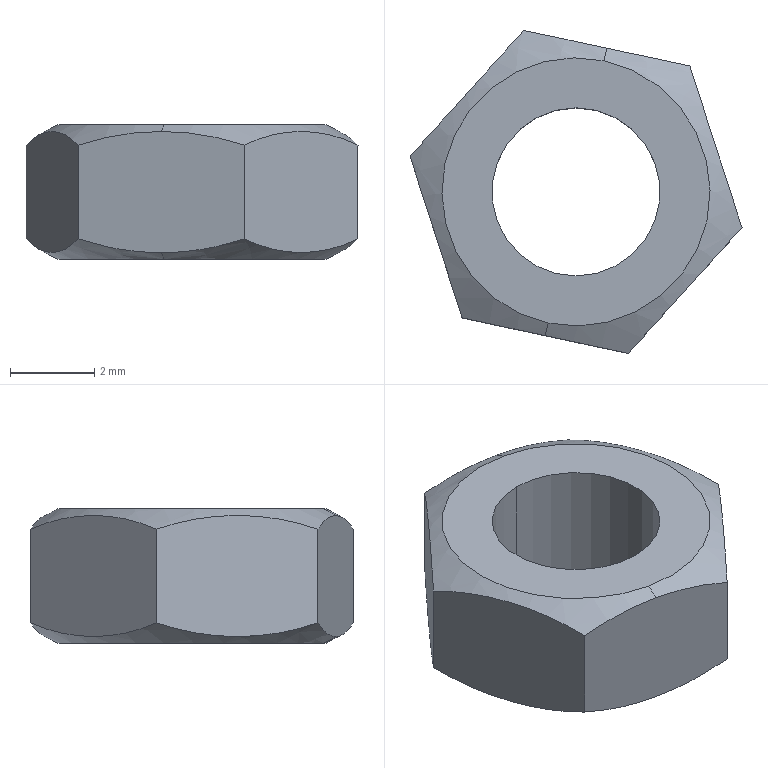Part | STEP file | MSBR-12_1_1_1_1 | 1 solid | 14 faces | box 7.904 x 7.691 x 3.2 mm | volume 92.564 mm3 | plane 8 | sphere 4 | cylinder 2 | commonest cylinder face diameters 4 x2
STEP:
#1=CARTESIAN_POINT('',(0.,0.,0.));
#2=DIRECTION('',(0.,0.,1.));
#3=DIRECTION('',(1.,0.,0.));
#4=AXIS2_PLACEMENT_3D('',#1,#2,#3);
#5=CARTESIAN_POINT('',(-32.173,30.173,38.8));
#6=VERTEX_POINT('',#5);
#7=CARTESIAN_POINT('',(-32.173,30.173,35.6));
#8=VERTEX_POINT('',#7);
#9=CARTESIAN_POINT('',(-32.173,30.173,38.8));
#10=DIRECTION('',(0.,0.,-1.));
#11=VECTOR('',#10,3.2);
#12=LINE('',#9,#11);
#13=EDGE_CURVE('',#6,#8,#12,.T.);
#14=ORIENTED_EDGE('',*,*,#13,.F.);
#15=CARTESIAN_POINT('',(-32.173,34.173,38.8));
#16=VERTEX_POINT('',#15);
#17=CARTESIAN_POINT('',(-32.173,32.173,38.8));
#18=DIRECTION('',(0.,0.,1.));
#19=DIRECTION('',(0.,1.,0.));
#20=AXIS2_PLACEMENT_3D('',#17,#18,#19);
#21=CIRCLE('',#20,2.);
#22=EDGE_CURVE('',#16,#6,#21,.T.);
#23=ORIENTED_EDGE('',*,*,#22,.F.);
#24=CARTESIAN_POINT('',(-32.173,34.173,35.6));
#25=VERTEX_POINT('',#24);
#26=CARTESIAN_POINT('',(-32.173,34.173,35.6));
#27=DIRECTION('',(0.,0.,1.));
#28=VECTOR('',#27,3.2);
#29=LINE('',#26,#28);
#30=EDGE_CURVE('',#25,#16,#29,.T.);
#31=ORIENTED_EDGE('',*,*,#30,.F.);
#32=CARTESIAN_POINT('',(-32.173,32.173,35.6));
#33=DIRECTION('',(0.,0.,-1.));
#34=DIRECTION('',(0.,-1.,0.));
#35=AXIS2_PLACEMENT_3D('',#32,#33,#34);
#36=CIRCLE('',#35,2.);
#37=EDGE_CURVE('',#8,#25,#36,.T.);
#38=ORIENTED_EDGE('',*,*,#37,.F.);
#39=EDGE_LOOP('',(#14,#23,#31,#38));
#40=FACE_OUTER_BOUND('',#39,.F.);
#41=CARTESIAN_POINT('',(-32.173,32.173,35.536));
#42=DIRECTION('',(0.,0.,1.));
#43=DIRECTION('',(0.,1.,0.));
#44=AXIS2_PLACEMENT_3D('',#41,#42,#43);
#45=CYLINDRICAL_SURFACE('',#44,2.);
#46=ADVANCED_FACE('',(#40),#45,.F.);
#47=CARTESIAN_POINT('',(-32.173,32.173,38.8));
#48=DIRECTION('',(0.,0.,1.));
#49=DIRECTION('',(0.,-1.,0.));
#50=AXIS2_PLACEMENT_3D('',#47,#48,#49);
#51=CIRCLE('',#50,2.);
#52=EDGE_CURVE('',#6,#16,#51,.T.);
#53=ORIENTED_EDGE('',*,*,#52,.F.);
#54=ORIENTED_EDGE('',*,*,#13,.T.);
#55=CARTESIAN_POINT('',(-32.173,32.173,35.6));
#56=DIRECTION('',(0.,0.,-1.));
#57=DIRECTION('',(0.,1.,0.));
#58=AXIS2_PLACEMENT_3D('',#55,#56,#57);
#59=CIRCLE('',#58,2.);
#60=EDGE_CURVE('',#25,#8,#59,.T.);
#61=ORIENTED_EDGE('',*,*,#60,.F.);
#62=ORIENTED_EDGE('',*,*,#30,.T.);
#63=EDGE_LOOP('',(#53,#54,#61,#62));
#64=FACE_OUTER_BOUND('',#63,.F.);
#65=CARTESIAN_POINT('',(-32.173,32.173,35.536));
#66=DIRECTION('',(0.,0.,1.));
#67=DIRECTION('',(0.,-1.,0.));
#68=AXIS2_PLACEMENT_3D('',#65,#66,#67);
#69=CYLINDRICAL_SURFACE('',#68,2.);
#70=ADVANCED_FACE('',(#64),#69,.F.);
#71=CARTESIAN_POINT('',(-32.842,29.052,38.8));
#72=VERTEX_POINT('',#71);
#73=CARTESIAN_POINT('',(-31.505,35.295,38.8));
#74=VERTEX_POINT('',#73);
#75=CARTESIAN_POINT('',(-32.173,32.173,38.8));
#76=DIRECTION('',(0.,0.,1.));
#77=DIRECTION('',(-0.2094,-0.9778,0.));
#78=AXIS2_PLACEMENT_3D('',#75,#76,#77);
#79=CIRCLE('',#78,3.192);
#80=EDGE_CURVE('',#72,#74,#79,.T.);
#81=ORIENTED_EDGE('',*,*,#80,.F.);
#82=CARTESIAN_POINT('',(-32.173,32.173,38.8));
#83=DIRECTION('',(0.,0.,-1.));
#84=DIRECTION('',(-0.2094,-0.9778,0.));
#85=AXIS2_PLACEMENT_3D('',#82,#83,#84);
#86=CIRCLE('',#85,3.192);
#87=EDGE_CURVE('',#72,#74,#86,.T.);
#88=ORIENTED_EDGE('',*,*,#87,.T.);
#89=EDGE_LOOP('',(#81,#88));
#90=FACE_OUTER_BOUND('',#89,.F.);
#91=ORIENTED_EDGE('',*,*,#22,.T.);
#92=ORIENTED_EDGE('',*,*,#52,.T.);
#93=EDGE_LOOP('',(#91,#92));
#94=FACE_BOUND('',#93,.F.);
#95=CARTESIAN_POINT('',(-32.173,32.173,38.8));
#96=DIRECTION('',(0.,0.,1.));
#97=DIRECTION('',(0.9778,-0.2094,0.));
#98=AXIS2_PLACEMENT_3D('',#95,#96,#97);
#99=PLANE('',#98);
#100=ADVANCED_FACE('',(#90,#94),#99,.T.);
#101=CARTESIAN_POINT('',(-32.906,28.751,38.641));
#102=VERTEX_POINT('',#101);
#103=CARTESIAN_POINT('',(-32.173,32.173,32.235));
#104=DIRECTION('',(0.9778,-0.2094,-0.000000001));
#105=DIRECTION('',(-0.09156,-0.4276,0.8993));
#106=AXIS2_PLACEMENT_3D('',#103,#104,#105);
#107=CIRCLE('',#106,7.3);
#108=EDGE_CURVE('',#72,#102,#107,.T.);
#109=ORIENTED_EDGE('',*,*,#108,.F.);
#110=ORIENTED_EDGE('',*,*,#80,.T.);
#111=CARTESIAN_POINT('',(-31.44,35.596,38.641));
#112=VERTEX_POINT('',#111);
#113=CARTESIAN_POINT('',(-32.173,32.173,32.235));
#114=DIRECTION('',(0.9778,-0.2094,-0.000000001));
#115=DIRECTION('',(0.1004,0.4688,0.8776));
#116=AXIS2_PLACEMENT_3D('',#113,#114,#115);
#117=CIRCLE('',#116,7.3);
#118=EDGE_CURVE('',#112,#74,#117,.T.);
#119=ORIENTED_EDGE('',*,*,#118,.F.);
#120=CARTESIAN_POINT('',(-29.465,35.173,38.314));
#121=VERTEX_POINT('',#120);
#122=CARTESIAN_POINT('',(-31.44,35.596,32.235));
#123=DIRECTION('',(0.2094,0.9778,0.));
#124=DIRECTION('',(-0.000000002,0.,1.));
#125=AXIS2_PLACEMENT_3D('',#122,#123,#124);
#126=CIRCLE('',#125,6.406);
#127=EDGE_CURVE('',#112,#121,#126,.T.);
#128=ORIENTED_EDGE('',*,*,#127,.T.);
#129=CARTESIAN_POINT('',(-28.222,31.327,38.314));
#130=VERTEX_POINT('',#129);
#131=CARTESIAN_POINT('',(-28.843,33.25,32.235));
#132=DIRECTION('',(0.9515,0.3076,0.));
#133=DIRECTION('',(-0.09701,0.3001,0.9489));
#134=AXIS2_PLACEMENT_3D('',#131,#132,#133);
#135=CIRCLE('',#134,6.406);
#136=EDGE_CURVE('',#121,#130,#135,.T.);
#137=ORIENTED_EDGE('',*,*,#136,.T.);
#138=CARTESIAN_POINT('',(-30.93,28.328,38.314));
#139=VERTEX_POINT('',#138);
#140=CARTESIAN_POINT('',(-29.576,29.827,32.235));
#141=DIRECTION('',(0.7421,-0.6703,0.));
#142=DIRECTION('',(0.2114,0.2341,0.9489));
#143=AXIS2_PLACEMENT_3D('',#140,#141,#142);
#144=CIRCLE('',#143,6.406);
#145=EDGE_CURVE('',#130,#139,#144,.T.);
#146=ORIENTED_EDGE('',*,*,#145,.T.);
#147=CARTESIAN_POINT('',(-32.906,28.751,32.235));
#148=DIRECTION('',(0.2094,0.9778,0.));
#149=DIRECTION('',(-0.000000001,0.,1.));
#150=AXIS2_PLACEMENT_3D('',#147,#148,#149);
#151=CIRCLE('',#150,6.406);
#152=EDGE_CURVE('',#102,#139,#151,.T.);
#153=ORIENTED_EDGE('',*,*,#152,.F.);
#154=EDGE_LOOP('',(#109,#110,#119,#128,#137,#146,#153));
#155=FACE_OUTER_BOUND('',#154,.F.);
#156=CARTESIAN_POINT('',(-32.173,32.173,32.235));
#157=DIRECTION('',(0.09156,0.4276,0.8993));
#158=DIRECTION('',(-0.1883,-0.8794,0.4373));
#159=AXIS2_PLACEMENT_3D('',#156,#157,#158);
#160=SPHERICAL_SURFACE('',#159,7.3);
#161=ADVANCED_FACE('',(#155),#160,.T.);
#162=CARTESIAN_POINT('',(-34.882,29.174,38.314));
#163=VERTEX_POINT('',#162);
#164=CARTESIAN_POINT('',(-32.906,28.751,32.235));
#165=DIRECTION('',(0.2094,0.9778,0.));
#166=DIRECTION('',(-0.3084,0.06605,0.9489));
#167=AXIS2_PLACEMENT_3D('',#164,#165,#166);
#168=CIRCLE('',#167,6.406);
#169=EDGE_CURVE('',#163,#102,#168,.T.);
#170=ORIENTED_EDGE('',*,*,#169,.F.);
#171=CARTESIAN_POINT('',(-36.125,33.02,38.314));
#172=VERTEX_POINT('',#171);
#173=CARTESIAN_POINT('',(-35.504,31.097,32.235));
#174=DIRECTION('',(-0.9515,-0.3076,0.));
#175=DIRECTION('',(0.09701,-0.3001,0.9489));
#176=AXIS2_PLACEMENT_3D('',#173,#174,#175);
#177=CIRCLE('',#176,6.406);
#178=EDGE_CURVE('',#163,#172,#177,.T.);
#179=ORIENTED_EDGE('',*,*,#178,.T.);
#180=CARTESIAN_POINT('',(-33.416,36.019,38.314));
#181=VERTEX_POINT('',#180);
#182=CARTESIAN_POINT('',(-34.771,34.519,32.235));
#183=DIRECTION('',(-0.7421,0.6703,0.));
#184=DIRECTION('',(-0.2114,-0.2341,0.9489));
#185=AXIS2_PLACEMENT_3D('',#182,#183,#184);
#186=CIRCLE('',#185,6.406);
#187=EDGE_CURVE('',#172,#181,#186,.T.);
#188=ORIENTED_EDGE('',*,*,#187,.T.);
#189=CARTESIAN_POINT('',(-31.44,35.596,32.235));
#190=DIRECTION('',(0.2094,0.9778,0.));
#191=DIRECTION('',(-0.3084,0.06605,0.9489));
#192=AXIS2_PLACEMENT_3D('',#189,#190,#191);
#193=CIRCLE('',#192,6.406);
#194=EDGE_CURVE('',#181,#112,#193,.T.);
#195=ORIENTED_EDGE('',*,*,#194,.T.);
#196=ORIENTED_EDGE('',*,*,#118,.T.);
#197=ORIENTED_EDGE('',*,*,#87,.F.);
#198=ORIENTED_EDGE('',*,*,#108,.T.);
#199=EDGE_LOOP('',(#170,#179,#188,#195,#196,#197,#198));
#200=FACE_OUTER_BOUND('',#199,.F.);
#201=CARTESIAN_POINT('',(-32.173,32.173,32.235));
#202=DIRECTION('',(0.09156,0.4276,0.8993));
#203=DIRECTION('',(0.1883,0.8794,-0.4373));
#204=AXIS2_PLACEMENT_3D('',#201,#202,#203);
#205=SPHERICAL_SURFACE('',#204,7.3);
#206=ADVANCED_FACE('',(#200),#205,.T.);
#207=ORIENTED_EDGE('',*,*,#152,.T.);
#208=CARTESIAN_POINT('',(-30.93,28.328,36.086));
#209=VERTEX_POINT('',#208);
#210=CARTESIAN_POINT('',(-30.93,28.328,36.086));
#211=DIRECTION('',(0.,0.,1.));
#212=VECTOR('',#211,2.228);
#213=LINE('',#210,#212);
#214=EDGE_CURVE('',#209,#139,#213,.T.);
#215=ORIENTED_EDGE('',*,*,#214,.F.);
#216=CARTESIAN_POINT('',(-32.906,28.751,35.759));
#217=VERTEX_POINT('',#216);
#218=CARTESIAN_POINT('',(-32.906,28.751,42.165));
#219=DIRECTION('',(-0.2094,-0.9778,0.));
#220=DIRECTION('',(-0.000000001,0.,-1.));
#221=AXIS2_PLACEMENT_3D('',#218,#219,#220);
#222=CIRCLE('',#221,6.406);
#223=EDGE_CURVE('',#217,#209,#222,.T.);
#224=ORIENTED_EDGE('',*,*,#223,.F.);
#225=CARTESIAN_POINT('',(-34.882,29.174,36.086));
#226=VERTEX_POINT('',#225);
#227=CARTESIAN_POINT('',(-32.906,28.751,42.165));
#228=DIRECTION('',(-0.2094,-0.9778,0.));
#229=DIRECTION('',(-0.3084,0.06605,-0.9489));
#230=AXIS2_PLACEMENT_3D('',#227,#228,#229);
#231=CIRCLE('',#230,6.406);
#232=EDGE_CURVE('',#226,#217,#231,.T.);
#233=ORIENTED_EDGE('',*,*,#232,.F.);
#234=CARTESIAN_POINT('',(-34.882,29.174,38.314));
#235=DIRECTION('',(0.,0.,-1.));
#236=VECTOR('',#235,2.228);
#237=LINE('',#234,#236);
#238=EDGE_CURVE('',#163,#226,#237,.T.);
#239=ORIENTED_EDGE('',*,*,#238,.F.);
#240=ORIENTED_EDGE('',*,*,#169,.T.);
#241=EDGE_LOOP('',(#207,#215,#224,#233,#239,#240));
#242=FACE_OUTER_BOUND('',#241,.F.);
#243=CARTESIAN_POINT('',(-32.906,28.751,37.2));
#244=DIRECTION('',(0.2094,0.9778,0.));
#245=DIRECTION('',(0.9778,-0.2094,0.));
#246=AXIS2_PLACEMENT_3D('',#243,#244,#245);
#247=PLANE('',#246);
#248=ADVANCED_FACE('',(#242),#247,.F.);
#249=ORIENTED_EDGE('',*,*,#145,.F.);
#250=CARTESIAN_POINT('',(-28.222,31.327,36.086));
#251=VERTEX_POINT('',#250);
#252=CARTESIAN_POINT('',(-28.222,31.327,36.086));
#253=DIRECTION('',(0.,0.,1.));
#254=VECTOR('',#253,2.228);
#255=LINE('',#252,#254);
#256=EDGE_CURVE('',#251,#130,#255,.T.);
#257=ORIENTED_EDGE('',*,*,#256,.F.);
#258=CARTESIAN_POINT('',(-29.576,29.827,42.165));
#259=DIRECTION('',(0.7421,-0.6703,0.));
#260=DIRECTION('',(-0.2114,-0.2341,-0.9489));
#261=AXIS2_PLACEMENT_3D('',#258,#259,#260);
#262=CIRCLE('',#261,6.406);
#263=EDGE_CURVE('',#209,#251,#262,.T.);
#264=ORIENTED_EDGE('',*,*,#263,.F.);
#265=ORIENTED_EDGE('',*,*,#214,.T.);
#266=EDGE_LOOP('',(#249,#257,#264,#265));
#267=FACE_OUTER_BOUND('',#266,.F.);
#268=CARTESIAN_POINT('',(-29.576,29.827,37.2));
#269=DIRECTION('',(0.7421,-0.6703,0.));
#270=DIRECTION('',(0.6703,0.7421,0.));
#271=AXIS2_PLACEMENT_3D('',#268,#269,#270);
#272=PLANE('',#271);
#273=ADVANCED_FACE('',(#267),#272,.T.);
#274=ORIENTED_EDGE('',*,*,#136,.F.);
#275=CARTESIAN_POINT('',(-29.465,35.173,36.086));
#276=VERTEX_POINT('',#275);
#277=CARTESIAN_POINT('',(-29.465,35.173,36.086));
#278=DIRECTION('',(0.,0.,1.));
#279=VECTOR('',#278,2.228);
#280=LINE('',#277,#279);
#281=EDGE_CURVE('',#276,#121,#280,.T.);
#282=ORIENTED_EDGE('',*,*,#281,.F.);
#283=CARTESIAN_POINT('',(-28.843,33.25,42.165));
#284=DIRECTION('',(0.9515,0.3076,0.));
#285=DIRECTION('',(0.09701,-0.3001,-0.9489));
#286=AXIS2_PLACEMENT_3D('',#283,#284,#285);
#287=CIRCLE('',#286,6.406);
#288=EDGE_CURVE('',#251,#276,#287,.T.);
#289=ORIENTED_EDGE('',*,*,#288,.F.);
#290=ORIENTED_EDGE('',*,*,#256,.T.);
#291=EDGE_LOOP('',(#274,#282,#289,#290));
#292=FACE_OUTER_BOUND('',#291,.F.);
#293=CARTESIAN_POINT('',(-28.843,33.25,37.2));
#294=DIRECTION('',(0.9515,0.3076,0.));
#295=DIRECTION('',(-0.3076,0.9515,0.));
#296=AXIS2_PLACEMENT_3D('',#293,#294,#295);
#297=PLANE('',#296);
#298=ADVANCED_FACE('',(#292),#297,.T.);
#299=ORIENTED_EDGE('',*,*,#281,.T.);
#300=ORIENTED_EDGE('',*,*,#127,.F.);
#301=ORIENTED_EDGE('',*,*,#194,.F.);
#302=CARTESIAN_POINT('',(-33.416,36.019,36.086));
#303=VERTEX_POINT('',#302);
#304=CARTESIAN_POINT('',(-33.416,36.019,36.086));
#305=DIRECTION('',(0.,0.,1.));
#306=VECTOR('',#305,2.228);
#307=LINE('',#304,#306);
#308=EDGE_CURVE('',#303,#181,#307,.T.);
#309=ORIENTED_EDGE('',*,*,#308,.F.);
#310=CARTESIAN_POINT('',(-31.44,35.596,35.759));
#311=VERTEX_POINT('',#310);
#312=CARTESIAN_POINT('',(-31.44,35.596,42.165));
#313=DIRECTION('',(-0.2094,-0.9778,0.));
#314=DIRECTION('',(-0.3084,0.06605,-0.9489));
#315=AXIS2_PLACEMENT_3D('',#312,#313,#314);
#316=CIRCLE('',#315,6.406);
#317=EDGE_CURVE('',#303,#311,#316,.T.);
#318=ORIENTED_EDGE('',*,*,#317,.T.);
#319=CARTESIAN_POINT('',(-31.44,35.596,42.165));
#320=DIRECTION('',(-0.2094,-0.9778,0.));
#321=DIRECTION('',(-0.000000001,0.,-1.));
#322=AXIS2_PLACEMENT_3D('',#319,#320,#321);
#323=CIRCLE('',#322,6.406);
#324=EDGE_CURVE('',#311,#276,#323,.T.);
#325=ORIENTED_EDGE('',*,*,#324,.T.);
#326=EDGE_LOOP('',(#299,#300,#301,#309,#318,#325));
#327=FACE_OUTER_BOUND('',#326,.F.);
#328=CARTESIAN_POINT('',(-31.44,35.596,37.2));
#329=DIRECTION('',(0.2094,0.9778,0.));
#330=DIRECTION('',(-0.9778,0.2094,0.));
#331=AXIS2_PLACEMENT_3D('',#328,#329,#330);
#332=PLANE('',#331);
#333=ADVANCED_FACE('',(#327),#332,.T.);
#334=CARTESIAN_POINT('',(-36.125,33.02,36.086));
#335=VERTEX_POINT('',#334);
#336=CARTESIAN_POINT('',(-34.771,34.519,42.165));
#337=DIRECTION('',(-0.7421,0.6703,0.));
#338=DIRECTION('',(0.2114,0.2341,-0.9489));
#339=AXIS2_PLACEMENT_3D('',#336,#337,#338);
#340=CIRCLE('',#339,6.406);
#341=EDGE_CURVE('',#303,#335,#340,.T.);
#342=ORIENTED_EDGE('',*,*,#341,.F.);
#343=ORIENTED_EDGE('',*,*,#308,.T.);
#344=ORIENTED_EDGE('',*,*,#187,.F.);
#345=CARTESIAN_POINT('',(-36.125,33.02,36.086));
#346=DIRECTION('',(0.,0.,1.));
#347=VECTOR('',#346,2.228);
#348=LINE('',#345,#347);
#349=EDGE_CURVE('',#335,#172,#348,.T.);
#350=ORIENTED_EDGE('',*,*,#349,.F.);
#351=EDGE_LOOP('',(#342,#343,#344,#350));
#352=FACE_OUTER_BOUND('',#351,.F.);
#353=CARTESIAN_POINT('',(-34.771,34.519,37.2));
#354=DIRECTION('',(0.7421,-0.6703,0.));
#355=DIRECTION('',(-0.6703,-0.7421,0.));
#356=AXIS2_PLACEMENT_3D('',#353,#354,#355);
#357=PLANE('',#356);
#358=ADVANCED_FACE('',(#352),#357,.F.);
#359=CARTESIAN_POINT('',(-32.842,29.052,35.6));
#360=VERTEX_POINT('',#359);
#361=CARTESIAN_POINT('',(-31.505,35.295,35.6));
#362=VERTEX_POINT('',#361);
#363=CARTESIAN_POINT('',(-32.173,32.173,35.6));
#364=DIRECTION('',(0.,0.,-1.));
#365=DIRECTION('',(-0.2094,-0.9778,0.));
#366=AXIS2_PLACEMENT_3D('',#363,#364,#365);
#367=CIRCLE('',#366,3.192);
#368=EDGE_CURVE('',#360,#362,#367,.T.);
#369=ORIENTED_EDGE('',*,*,#368,.T.);
#370=CARTESIAN_POINT('',(-32.173,32.173,42.165));
#371=DIRECTION('',(-0.9778,0.2094,0.000000001));
#372=DIRECTION('',(0.1004,0.4688,-0.8776));
#373=AXIS2_PLACEMENT_3D('',#370,#371,#372);
#374=CIRCLE('',#373,7.3);
#375=EDGE_CURVE('',#311,#362,#374,.T.);
#376=ORIENTED_EDGE('',*,*,#375,.F.);
#377=ORIENTED_EDGE('',*,*,#317,.F.);
#378=ORIENTED_EDGE('',*,*,#341,.T.);
#379=CARTESIAN_POINT('',(-35.504,31.097,42.165));
#380=DIRECTION('',(-0.9515,-0.3076,0.));
#381=DIRECTION('',(-0.09701,0.3001,-0.9489));
#382=AXIS2_PLACEMENT_3D('',#379,#380,#381);
#383=CIRCLE('',#382,6.406);
#384=EDGE_CURVE('',#335,#226,#383,.T.);
#385=ORIENTED_EDGE('',*,*,#384,.T.);
#386=ORIENTED_EDGE('',*,*,#232,.T.);
#387=CARTESIAN_POINT('',(-32.173,32.173,42.165));
#388=DIRECTION('',(-0.9778,0.2094,0.000000005));
#389=DIRECTION('',(-0.09156,-0.4276,-0.8993));
#390=AXIS2_PLACEMENT_3D('',#387,#388,#389);
#391=CIRCLE('',#390,7.3);
#392=EDGE_CURVE('',#360,#217,#391,.T.);
#393=ORIENTED_EDGE('',*,*,#392,.F.);
#394=EDGE_LOOP('',(#369,#376,#377,#378,#385,#386,#393));
#395=FACE_OUTER_BOUND('',#394,.F.);
#396=CARTESIAN_POINT('',(-32.173,32.173,42.165));
#397=DIRECTION('',(-0.09156,-0.4276,-0.8993));
#398=DIRECTION('',(-0.1883,-0.8794,0.4373));
#399=AXIS2_PLACEMENT_3D('',#396,#397,#398);
#400=SPHERICAL_SURFACE('',#399,7.3);
#401=ADVANCED_FACE('',(#395),#400,.T.);
#402=ORIENTED_EDGE('',*,*,#368,.F.);
#403=CARTESIAN_POINT('',(-32.173,32.173,35.6));
#404=DIRECTION('',(0.,0.,1.));
#405=DIRECTION('',(-0.2094,-0.9778,0.));
#406=AXIS2_PLACEMENT_3D('',#403,#404,#405);
#407=CIRCLE('',#406,3.192);
#408=EDGE_CURVE('',#360,#362,#407,.T.);
#409=ORIENTED_EDGE('',*,*,#408,.T.);
#410=EDGE_LOOP('',(#402,#409));
#411=FACE_OUTER_BOUND('',#410,.F.);
#412=ORIENTED_EDGE('',*,*,#60,.T.);
#413=ORIENTED_EDGE('',*,*,#37,.T.);
#414=EDGE_LOOP('',(#412,#413));
#415=FACE_BOUND('',#414,.F.);
#416=CARTESIAN_POINT('',(-32.173,32.173,35.6));
#417=DIRECTION('',(0.,0.,1.));
#418=DIRECTION('',(0.9778,-0.2094,0.));
#419=AXIS2_PLACEMENT_3D('',#416,#417,#418);
#420=PLANE('',#419);
#421=ADVANCED_FACE('',(#411,#415),#420,.F.);
#422=ORIENTED_EDGE('',*,*,#392,.T.);
#423=ORIENTED_EDGE('',*,*,#223,.T.);
#424=ORIENTED_EDGE('',*,*,#263,.T.);
#425=ORIENTED_EDGE('',*,*,#288,.T.);
#426=ORIENTED_EDGE('',*,*,#324,.F.);
#427=ORIENTED_EDGE('',*,*,#375,.T.);
#428=ORIENTED_EDGE('',*,*,#408,.F.);
#429=EDGE_LOOP('',(#422,#423,#424,#425,#426,#427,#428));
#430=FACE_OUTER_BOUND('',#429,.F.);
#431=CARTESIAN_POINT('',(-32.173,32.173,42.165));
#432=DIRECTION('',(-0.09156,-0.4276,-0.8993));
#433=DIRECTION('',(0.1883,0.8794,-0.4373));
#434=AXIS2_PLACEMENT_3D('',#431,#432,#433);
#435=SPHERICAL_SURFACE('',#434,7.3);
#436=ADVANCED_FACE('',(#430),#435,.T.);
#437=ORIENTED_EDGE('',*,*,#384,.F.);
#438=ORIENTED_EDGE('',*,*,#349,.T.);
#439=ORIENTED_EDGE('',*,*,#178,.F.);
#440=ORIENTED_EDGE('',*,*,#238,.T.);
#441=EDGE_LOOP('',(#437,#438,#439,#440));
#442=FACE_OUTER_BOUND('',#441,.F.);
#443=CARTESIAN_POINT('',(-35.504,31.097,37.2));
#444=DIRECTION('',(0.9515,0.3076,0.));
#445=DIRECTION('',(0.3076,-0.9515,0.));
#446=AXIS2_PLACEMENT_3D('',#443,#444,#445);
#447=PLANE('',#446);
#448=ADVANCED_FACE('',(#442),#447,.F.);
#449=CLOSED_SHELL('',(#46,#70,#100,#161,#206,#248,#273,#298,#333,#358,#401,#421,#436,#448));
#450=MANIFOLD_SOLID_BREP('',#449);
#451=(LENGTH_UNIT()NAMED_UNIT(*)SI_UNIT(.MILLI.,.METRE.));
#452=UNCERTAINTY_MEASURE_WITH_UNIT(LENGTH_MEASURE(0.00211),#451,'','');
#453=(NAMED_UNIT(*)PLANE_ANGLE_UNIT()SI_UNIT($,.RADIAN.));
#454=PLANE_ANGLE_MEASURE_WITH_UNIT(PLANE_ANGLE_MEASURE(0.01745),#453);
#455=(CONVERSION_BASED_UNIT('DEGREE',#454)NAMED_UNIT(*)PLANE_ANGLE_UNIT());
#456=(NAMED_UNIT(*)SI_UNIT($,.STERADIAN.)SOLID_ANGLE_UNIT());
#457=(GEOMETRIC_REPRESENTATION_CONTEXT(3)GLOBAL_UNCERTAINTY_ASSIGNED_CONTEXT((#452))GLOBAL_UNIT_ASSIGNED_CONTEXT((#451,#455,#456))REPRESENTATION_CONTEXT('',''));
#458=ADVANCED_BREP_SHAPE_REPRESENTATION('',(#4,#450),#457);